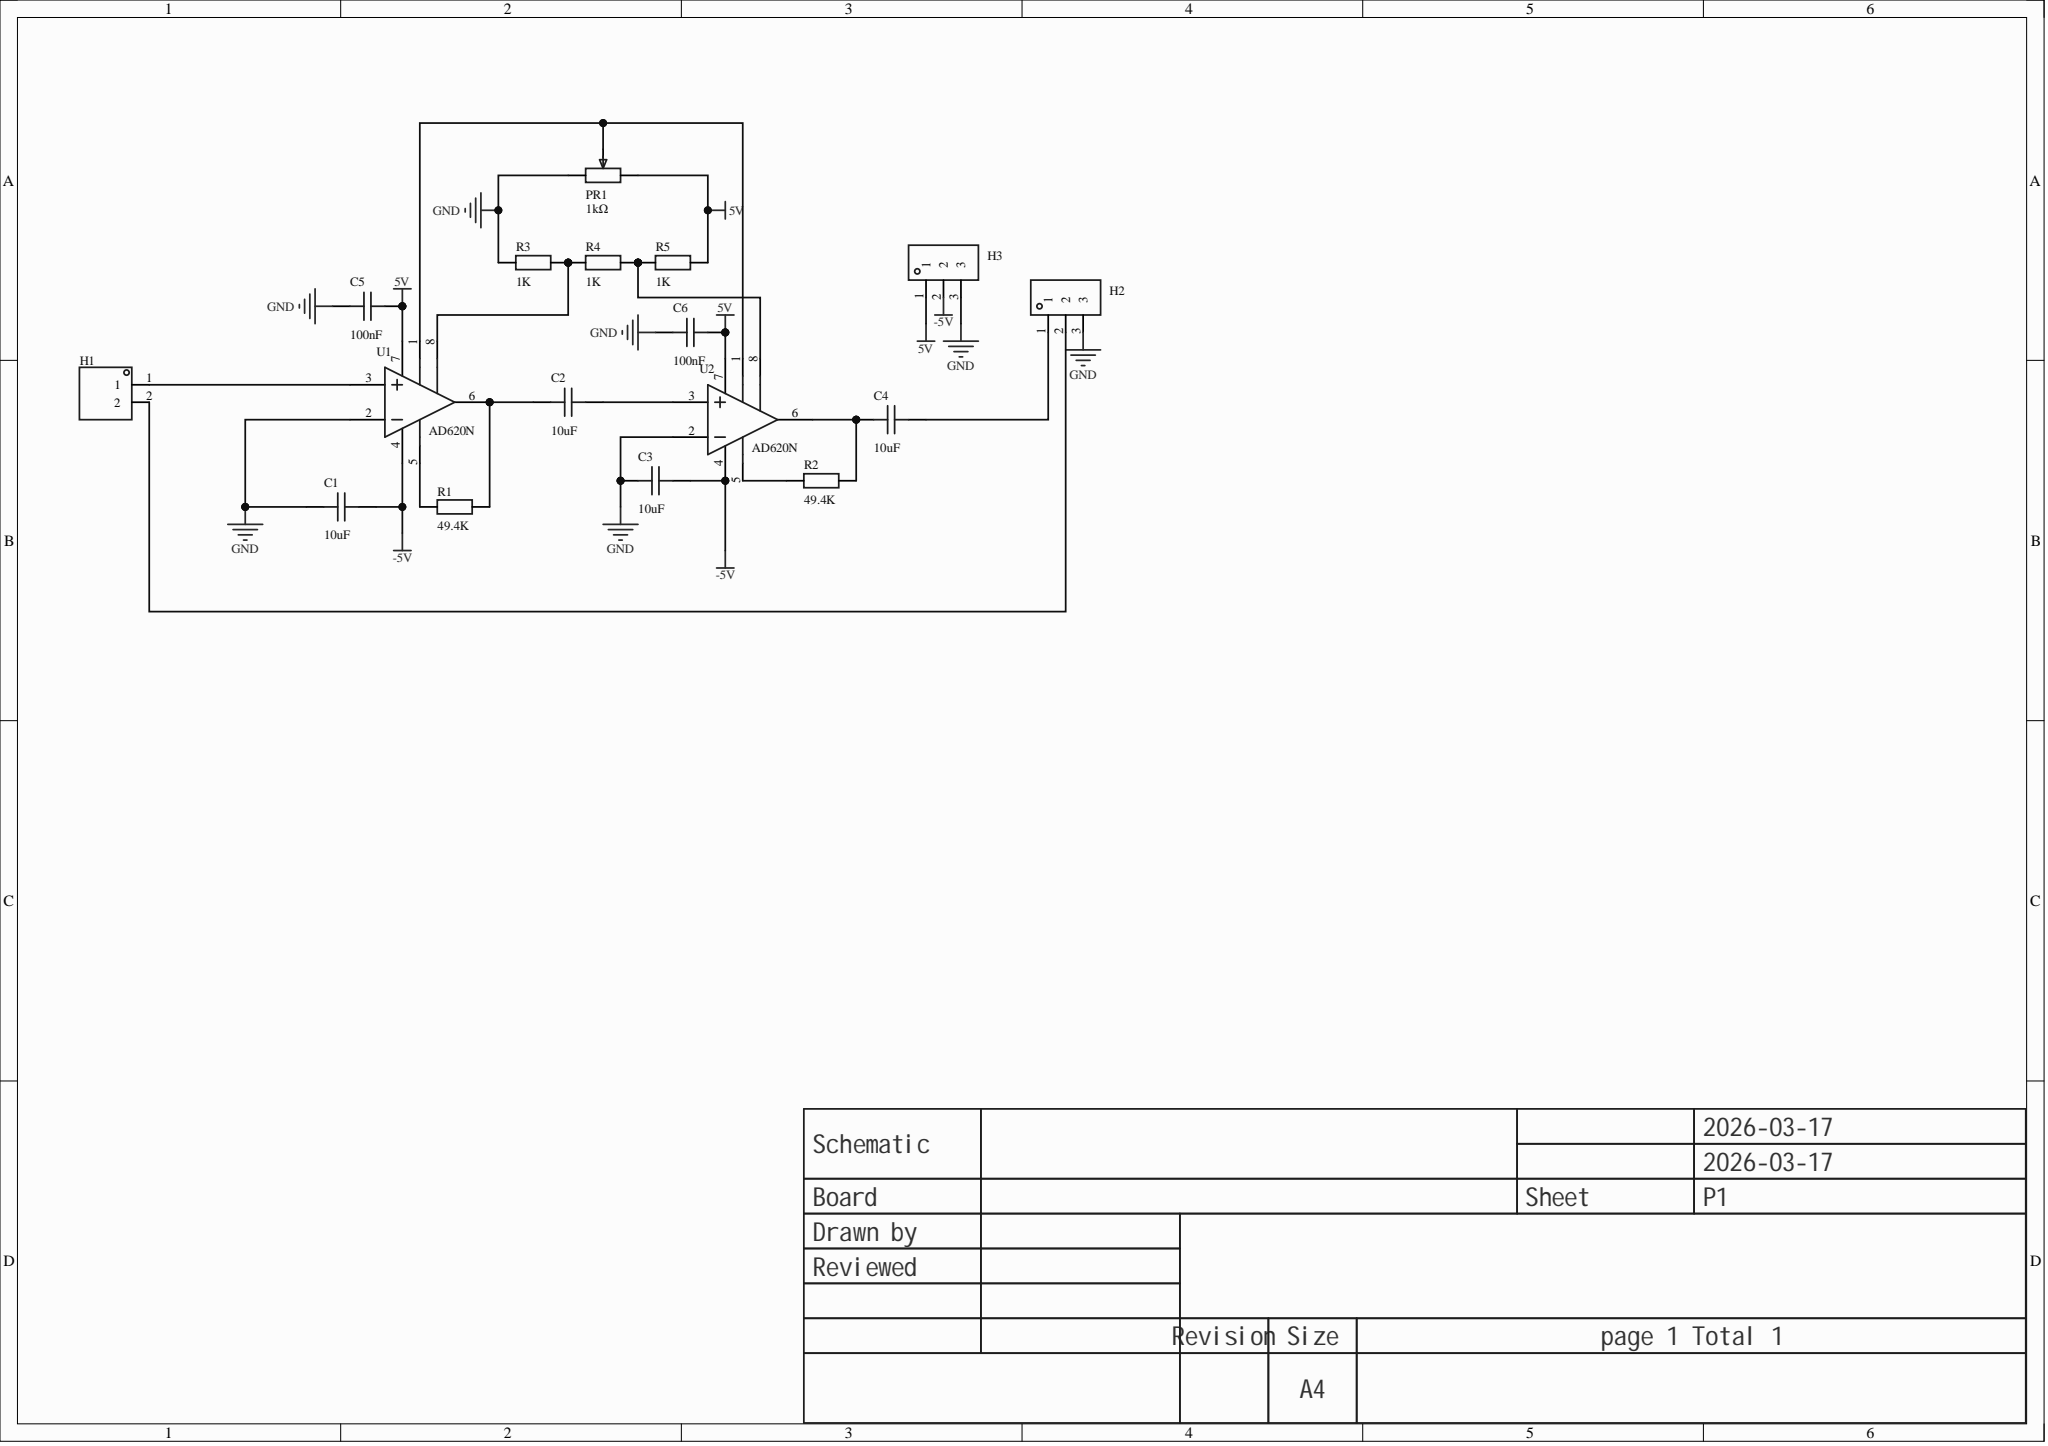Circuit board | Altium Designer | 17 parts | 14 nets
Bill of materials:
Comment,Description,Designator,Footprint,LibRef,Quantity
"10uF","","C1, C2, C3, C4","C0603","CAP_0603","4"
"100nF","","C5, C6","C0603","CAP_0603","2"
"","","H1","HDR-TH_2P-P2.54-V-M-1","HDR-M_2.54_1x2P","1"
"","","H2, H3","HDR-TH_3P-P2.54-V-M","HDR-M_2.54_1x3P","2"
"1kΩ","","PR1","R_3296","R_3296","1"
"49.4K","","R1, R2","R0603","Res_0603","2"
"1K","","R3, R4, R5","R0603","Res_0603","3"
"AD620N","Low-drift, low-power instrumentation amplifier, gain setting range 1 to 10000","U1, U2","SOIC-8_L5.0-W4.0-P1.27-LS6.0-BL","AD620BRZ-RL-JSM","2"
Netlist (Protel format):
[
C1
C0603
10uF



]
[
C2
C0603
10uF



]
[
C3
C0603
10uF



]
[
C4
C0603
10uF



]
[
C5
C0603
100nF



]
[
C6
C0603
100nF



]
[
H1
HDR-TH_2P-P2.54-V-M-1




]
[
H2
HDR-TH_3P-P2.54-V-M




]
[
H3
HDR-TH_3P-P2.54-V-M




]
[
PR1
R_3296
1kΩ



]
[
R1
R0603
49.4K



]
[
R2
R0603
49.4K



]
[
R3
R0603
1K



]
[
R4
R0603
1K



]
[
R5
R0603
1K



]
[
U1
SOIC-8_L5.0-W4.0-P1.27-LS6.0-BL
AD620N



]
[
U2
SOIC-8_L5.0-W4.0-P1.27-LS6.0-BL
AD620N



]
(
NetR4_2
R4-2
R5-1
U2-8
)
(
NetR3_2
R3-2
R4-1
U1-8
)
(
NetR2_1
R2-1
U2-5
)
(
NetR1_1
R1-1
U1-5
)
(
NetPR1_2
PR1-2
U1-1
U2-1
)
(
NetH1_2
H1-2
H2-2
)
(
NetH1_1
H1-1
U1-3
)
(
NetC4_2
C4-2
H2-1
)
(
NetC4_1
C4-1
R2-2
U2-6
)
(
NetC2_2
C2-2
U2-3
)
(
NetC2_1
C2-1
R1-2
U1-6
)
(
GND
C1-1
C3-1
C5-1
C6-1
H2-3
H3-3
PR1-3
R3-1
U1-2
U2-2
)
(
-5V
C1-2
C3-2
H3-2
U1-4
U2-4
)
(
5V
C5-2
C6-2
H3-1
PR1-1
R5-2
U1-7
U2-7
)